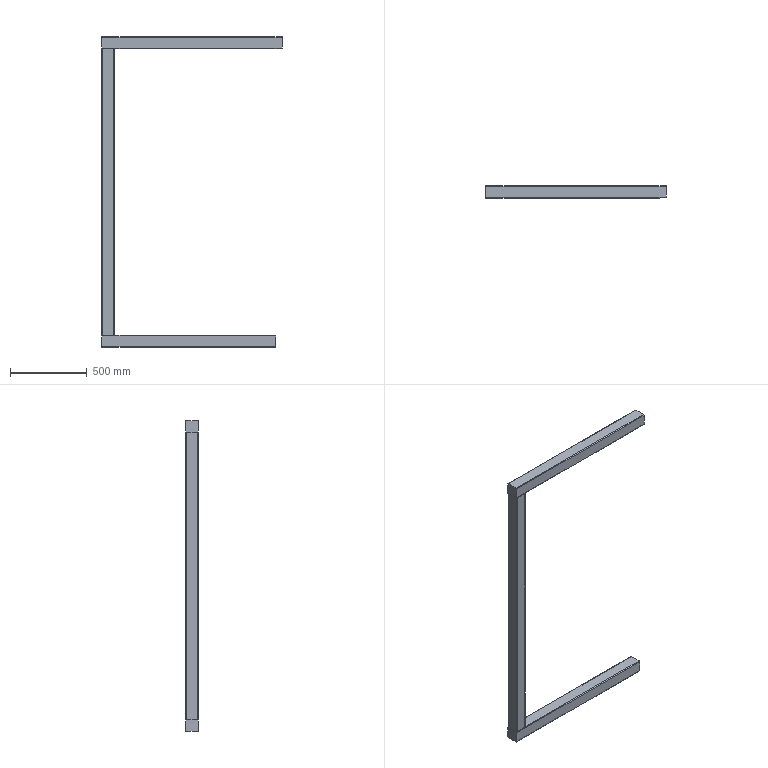Part | STEP file | Gantry | 3 solids | 38 faces | box 1171 x 80 x 2022 mm | volume 26562153 mm3 | cylinder 20 | plane 18 | commonest cylinder face diameters 10 x20